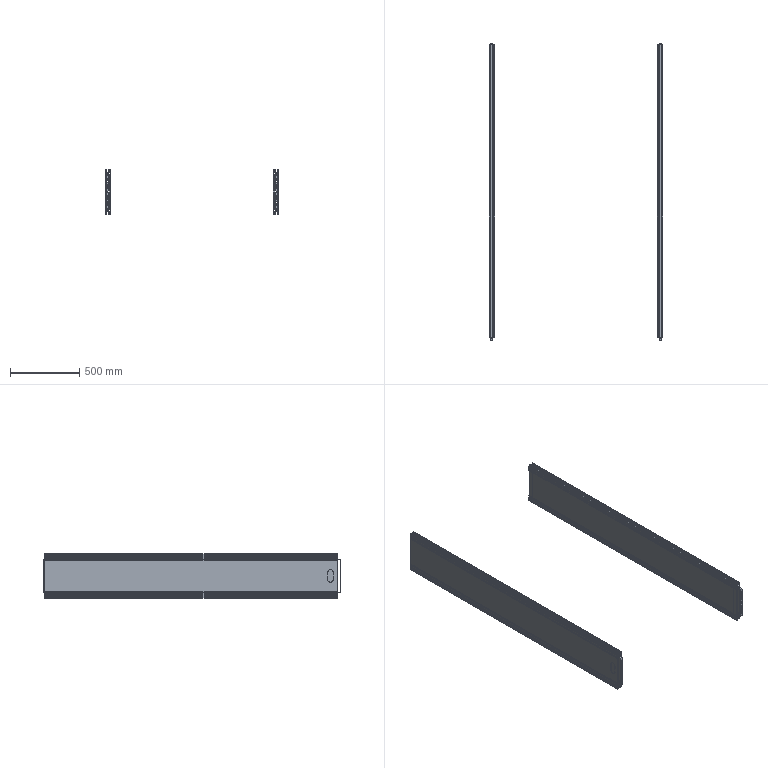Part | SolidWorks | features ReferencePattern 11, MirrorCompFeat 3 | 49 solids | 1341 faces | box 1250 x 2151 x 320 mm | volume 8404341 mm3 | plane 802 | cylinder 539 | commonest cylinder face diameters 8.5 x80 6 x72 8 x56 6.2 x48 8.2 x48 12 x48